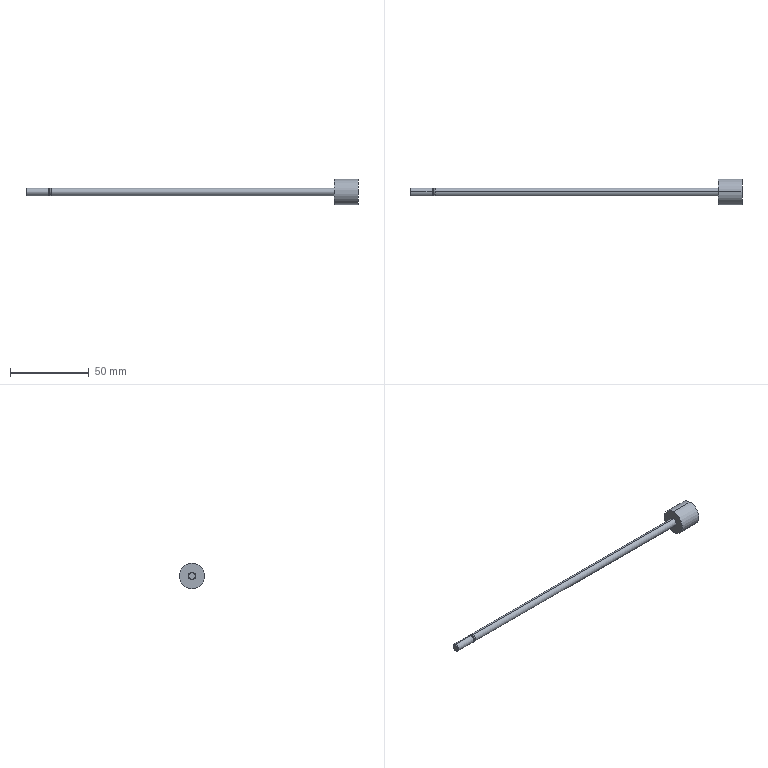Part | STEP file | QA-HI_SBA16x150-LB_R | 1 solid | 16 faces | box 210.5 x 16 x 16 mm | volume 6843 mm3 | cylinder 8 | cone 4 | plane 4 | commonest cylinder face diameters 5 x4 4 x2 16 x2
STEP:
#1=CARTESIAN_POINT('',(0.,0.,0.));
#2=DIRECTION('',(0.,0.,1.));
#3=DIRECTION('',(1.,0.,0.));
#4=AXIS2_PLACEMENT_3D('',#1,#2,#3);
#5=CARTESIAN_POINT('',(175.5,0.,2.5));
#6=VERTEX_POINT('',#5);
#7=CARTESIAN_POINT('',(175.5,0.,-2.5));
#8=VERTEX_POINT('',#7);
#9=CARTESIAN_POINT('',(175.5,0.,0.));
#10=DIRECTION('',(-1.,0.,0.));
#11=DIRECTION('',(0.,0.,1.));
#12=AXIS2_PLACEMENT_3D('',#9,#10,#11);
#13=CIRCLE('',#12,2.5);
#14=CARTESIAN_POINT('',(190.5,0.,0.));
#15=DIRECTION('',(-1.,0.,0.));
#16=DIRECTION('',(0.,0.,1.));
#17=AXIS2_PLACEMENT_3D('',#14,#15,#16);
#18=CYLINDRICAL_SURFACE('',#17,2.5);
#19=CARTESIAN_POINT('',(0.,15.));
#20=DIRECTION('',(1.,0.));
#21=VECTOR('',#20,1.);
#22=LINE('',#19,#21);
#23=(GEOMETRIC_REPRESENTATION_CONTEXT(2)PARAMETRIC_REPRESENTATION_CONTEXT()REPRESENTATION_CONTEXT('',''));
#24=DEFINITIONAL_REPRESENTATION('',(#22),#23);
#25=PCURVE('',#18,#24);
#26=CARTESIAN_POINT('',(175.5,2.5,0.));
#27=DIRECTION('',(1.,0.,0.));
#28=DIRECTION('',(0.,0.,-1.));
#29=AXIS2_PLACEMENT_3D('',#26,#27,#28);
#30=PLANE('',#29);
#31=CARTESIAN_POINT('',(-2.5,-2.5));
#32=CARTESIAN_POINT('',(-2.5,1.83));
#33=CARTESIAN_POINT('',(1.25,-0.3349));
#34=CARTESIAN_POINT('',(5.,-2.5));
#35=CARTESIAN_POINT('',(1.25,-4.665));
#36=CARTESIAN_POINT('',(-2.5,-6.83));
#37=CARTESIAN_POINT('',(-2.5,-2.5));
#38=(BOUNDED_CURVE()B_SPLINE_CURVE(2,(#31,#32,#33,#34,#35,#36,#37),.UNSPECIFIED.,.T.,.F.)B_SPLINE_CURVE_WITH_KNOTS((1,2,2,2,2,1),(-2.094,0.,2.094,4.189,6.283,8.378),.UNSPECIFIED.)CURVE()GEOMETRIC_REPRESENTATION_ITEM()RATIONAL_B_SPLINE_CURVE((1.,0.5,1.,0.5,1.,0.5,1.))REPRESENTATION_ITEM(''));
#39=(GEOMETRIC_REPRESENTATION_CONTEXT(2)PARAMETRIC_REPRESENTATION_CONTEXT()REPRESENTATION_CONTEXT('',''));
#40=DEFINITIONAL_REPRESENTATION('',(#38),#39);
#41=PCURVE('',#30,#40);
#42=SURFACE_CURVE('',#13,(#25,#41),.PCURVE_S1.);
#43=EDGE_CURVE('',#6,#8,#42,.T.);
#44=ORIENTED_EDGE('',*,*,#43,.T.);
#45=CARTESIAN_POINT('',(-4.134,0.,-2.5));
#46=VERTEX_POINT('',#45);
#47=CARTESIAN_POINT('',(190.5,0.,-2.5));
#48=DIRECTION('',(-1.,0.,0.));
#49=VECTOR('',#48,1.);
#50=LINE('',#47,#49);
#51=CARTESIAN_POINT('',(3.142,0.));
#52=DIRECTION('',(0.,1.));
#53=VECTOR('',#52,1.);
#54=LINE('',#51,#53);
#55=(GEOMETRIC_REPRESENTATION_CONTEXT(2)PARAMETRIC_REPRESENTATION_CONTEXT()REPRESENTATION_CONTEXT('',''));
#56=DEFINITIONAL_REPRESENTATION('',(#54),#55);
#57=PCURVE('',#18,#56);
#58=CARTESIAN_POINT('',(190.5,0.,0.));
#59=DIRECTION('',(-1.,0.,0.));
#60=DIRECTION('',(0.,0.,1.));
#61=AXIS2_PLACEMENT_3D('',#58,#59,#60);
#62=CYLINDRICAL_SURFACE('',#61,2.5);
#63=CARTESIAN_POINT('',(3.142,0.));
#64=DIRECTION('',(0.,1.));
#65=VECTOR('',#64,1.);
#66=LINE('',#63,#65);
#67=(GEOMETRIC_REPRESENTATION_CONTEXT(2)PARAMETRIC_REPRESENTATION_CONTEXT()REPRESENTATION_CONTEXT('',''));
#68=DEFINITIONAL_REPRESENTATION('',(#66),#67);
#69=PCURVE('',#62,#68);
#70=SURFACE_CURVE('',#50,(#57,#69),.PCURVE_S1.);
#71=EDGE_CURVE('',#8,#46,#70,.T.);
#72=ORIENTED_EDGE('',*,*,#71,.T.);
#73=CARTESIAN_POINT('',(-4.134,0.,2.5));
#74=VERTEX_POINT('',#73);
#75=CARTESIAN_POINT('',(-4.134,0.,0.));
#76=DIRECTION('',(1.,0.,0.));
#77=DIRECTION('',(0.,0.,1.));
#78=AXIS2_PLACEMENT_3D('',#75,#76,#77);
#79=CIRCLE('',#78,2.5);
#80=CARTESIAN_POINT('',(6.283,194.634));
#81=DIRECTION('',(-1.,0.));
#82=VECTOR('',#81,1.);
#83=LINE('',#80,#82);
#84=(GEOMETRIC_REPRESENTATION_CONTEXT(2)PARAMETRIC_REPRESENTATION_CONTEXT()REPRESENTATION_CONTEXT('',''));
#85=DEFINITIONAL_REPRESENTATION('',(#83),#84);
#86=PCURVE('',#18,#85);
#87=CARTESIAN_POINT('',(-4.134,0.,0.));
#88=DIRECTION('',(1.,0.,0.));
#89=DIRECTION('',(0.,0.,-1.));
#90=AXIS2_PLACEMENT_3D('',#87,#88,#89);
#91=CONICAL_SURFACE('',#90,2.5,0.5236);
#92=CARTESIAN_POINT('',(-3.142,0.));
#93=DIRECTION('',(1.,0.));
#94=VECTOR('',#93,1.);
#95=LINE('',#92,#94);
#96=(GEOMETRIC_REPRESENTATION_CONTEXT(2)PARAMETRIC_REPRESENTATION_CONTEXT()REPRESENTATION_CONTEXT('',''));
#97=DEFINITIONAL_REPRESENTATION('',(#95),#96);
#98=PCURVE('',#91,#97);
#99=SURFACE_CURVE('',#79,(#86,#98),.PCURVE_S1.);
#100=EDGE_CURVE('',#46,#74,#99,.T.);
#101=ORIENTED_EDGE('',*,*,#100,.T.);
#102=CARTESIAN_POINT('',(190.5,0.,2.5));
#103=DIRECTION('',(-1.,0.,0.));
#104=VECTOR('',#103,1.);
#105=LINE('',#102,#104);
#106=CARTESIAN_POINT('',(0.,0.));
#107=DIRECTION('',(0.,1.));
#108=VECTOR('',#107,1.);
#109=LINE('',#106,#108);
#110=(GEOMETRIC_REPRESENTATION_CONTEXT(2)PARAMETRIC_REPRESENTATION_CONTEXT()REPRESENTATION_CONTEXT('',''));
#111=DEFINITIONAL_REPRESENTATION('',(#109),#110);
#112=PCURVE('',#18,#111);
#113=CARTESIAN_POINT('',(6.283,0.));
#114=DIRECTION('',(0.,1.));
#115=VECTOR('',#114,1.);
#116=LINE('',#113,#115);
#117=(GEOMETRIC_REPRESENTATION_CONTEXT(2)PARAMETRIC_REPRESENTATION_CONTEXT()REPRESENTATION_CONTEXT('',''));
#118=DEFINITIONAL_REPRESENTATION('',(#116),#117);
#119=PCURVE('',#62,#118);
#120=SURFACE_CURVE('',#105,(#112,#119),.PCURVE_S1.);
#121=EDGE_CURVE('',#6,#74,#120,.T.);
#122=ORIENTED_EDGE('',*,*,#121,.F.);
#123=EDGE_LOOP('',(#44,#72,#101,#122));
#124=FACE_BOUND('',#123,.T.);
#125=ADVANCED_FACE('',(#124),#18,.T.);
#126=CARTESIAN_POINT('',(-5.,0.,-2.));
#127=VERTEX_POINT('',#126);
#128=CARTESIAN_POINT('',(-5.,0.,2.));
#129=VERTEX_POINT('',#128);
#130=CARTESIAN_POINT('',(-5.,0.,0.));
#131=DIRECTION('',(1.,0.,0.));
#132=DIRECTION('',(0.,0.,-1.));
#133=AXIS2_PLACEMENT_3D('',#130,#131,#132);
#134=CIRCLE('',#133,2.);
#135=CARTESIAN_POINT('',(0.,-0.866));
#136=DIRECTION('',(1.,0.));
#137=VECTOR('',#136,1.);
#138=LINE('',#135,#137);
#139=(GEOMETRIC_REPRESENTATION_CONTEXT(2)PARAMETRIC_REPRESENTATION_CONTEXT()REPRESENTATION_CONTEXT('',''));
#140=DEFINITIONAL_REPRESENTATION('',(#138),#139);
#141=PCURVE('',#91,#140);
#142=CARTESIAN_POINT('',(0.,0.,0.));
#143=DIRECTION('',(-1.,0.,0.));
#144=DIRECTION('',(0.,0.,1.));
#145=AXIS2_PLACEMENT_3D('',#142,#143,#144);
#146=CYLINDRICAL_SURFACE('',#145,2.);
#147=CARTESIAN_POINT('',(3.142,5.));
#148=DIRECTION('',(-1.,0.));
#149=VECTOR('',#148,1.);
#150=LINE('',#147,#149);
#151=(GEOMETRIC_REPRESENTATION_CONTEXT(2)PARAMETRIC_REPRESENTATION_CONTEXT()REPRESENTATION_CONTEXT('',''));
#152=DEFINITIONAL_REPRESENTATION('',(#150),#151);
#153=PCURVE('',#146,#152);
#154=SURFACE_CURVE('',#134,(#141,#153),.PCURVE_S1.);
#155=EDGE_CURVE('',#127,#129,#154,.T.);
#156=ORIENTED_EDGE('',*,*,#155,.T.);
#157=CARTESIAN_POINT('',(-4.134,0.,2.5));
#158=DIRECTION('',(0.866,0.,0.5));
#159=VECTOR('',#158,1.);
#160=LINE('',#157,#159);
#161=CARTESIAN_POINT('',(3.142,0.));
#162=DIRECTION('',(0.,1.));
#163=VECTOR('',#162,1.);
#164=LINE('',#161,#163);
#165=(GEOMETRIC_REPRESENTATION_CONTEXT(2)PARAMETRIC_REPRESENTATION_CONTEXT()REPRESENTATION_CONTEXT('',''));
#166=DEFINITIONAL_REPRESENTATION('',(#164),#165);
#167=PCURVE('',#91,#166);
#168=CARTESIAN_POINT('',(-4.134,0.,0.));
#169=DIRECTION('',(1.,0.,0.));
#170=DIRECTION('',(0.,0.,-1.));
#171=AXIS2_PLACEMENT_3D('',#168,#169,#170);
#172=CONICAL_SURFACE('',#171,2.5,0.5236);
#173=CARTESIAN_POINT('',(3.142,0.));
#174=DIRECTION('',(0.,1.));
#175=VECTOR('',#174,1.);
#176=LINE('',#173,#175);
#177=(GEOMETRIC_REPRESENTATION_CONTEXT(2)PARAMETRIC_REPRESENTATION_CONTEXT()REPRESENTATION_CONTEXT('',''));
#178=DEFINITIONAL_REPRESENTATION('',(#176),#177);
#179=PCURVE('',#172,#178);
#180=SURFACE_CURVE('',#160,(#167,#179),.PCURVE_S1.);
#181=EDGE_CURVE('',#129,#74,#180,.T.);
#182=ORIENTED_EDGE('',*,*,#181,.T.);
#183=ORIENTED_EDGE('',*,*,#100,.F.);
#184=CARTESIAN_POINT('',(-4.134,0.,-2.5));
#185=DIRECTION('',(0.866,0.,-0.5));
#186=VECTOR('',#185,1.);
#187=LINE('',#184,#186);
#188=CARTESIAN_POINT('',(0.,0.));
#189=DIRECTION('',(0.,1.));
#190=VECTOR('',#189,1.);
#191=LINE('',#188,#190);
#192=(GEOMETRIC_REPRESENTATION_CONTEXT(2)PARAMETRIC_REPRESENTATION_CONTEXT()REPRESENTATION_CONTEXT('',''));
#193=DEFINITIONAL_REPRESENTATION('',(#191),#192);
#194=PCURVE('',#91,#193);
#195=CARTESIAN_POINT('',(6.283,0.));
#196=DIRECTION('',(0.,1.));
#197=VECTOR('',#196,1.);
#198=LINE('',#195,#197);
#199=(GEOMETRIC_REPRESENTATION_CONTEXT(2)PARAMETRIC_REPRESENTATION_CONTEXT()REPRESENTATION_CONTEXT('',''));
#200=DEFINITIONAL_REPRESENTATION('',(#198),#199);
#201=PCURVE('',#172,#200);
#202=SURFACE_CURVE('',#187,(#194,#201),.PCURVE_S1.);
#203=EDGE_CURVE('',#127,#46,#202,.T.);
#204=ORIENTED_EDGE('',*,*,#203,.F.);
#205=EDGE_LOOP('',(#156,#182,#183,#204));
#206=FACE_BOUND('',#205,.T.);
#207=ADVANCED_FACE('',(#206),#91,.T.);
#208=ORIENTED_EDGE('',*,*,#155,.F.);
#209=CARTESIAN_POINT('',(-6.,0.,-2.));
#210=VERTEX_POINT('',#209);
#211=CARTESIAN_POINT('',(0.,0.,-2.));
#212=DIRECTION('',(-1.,0.,0.));
#213=VECTOR('',#212,1.);
#214=LINE('',#211,#213);
#215=CARTESIAN_POINT('',(3.142,0.));
#216=DIRECTION('',(0.,1.));
#217=VECTOR('',#216,1.);
#218=LINE('',#215,#217);
#219=(GEOMETRIC_REPRESENTATION_CONTEXT(2)PARAMETRIC_REPRESENTATION_CONTEXT()REPRESENTATION_CONTEXT('',''));
#220=DEFINITIONAL_REPRESENTATION('',(#218),#219);
#221=PCURVE('',#146,#220);
#222=CARTESIAN_POINT('',(0.,0.,0.));
#223=DIRECTION('',(-1.,0.,0.));
#224=DIRECTION('',(0.,0.,1.));
#225=AXIS2_PLACEMENT_3D('',#222,#223,#224);
#226=CYLINDRICAL_SURFACE('',#225,2.);
#227=CARTESIAN_POINT('',(3.142,0.));
#228=DIRECTION('',(0.,1.));
#229=VECTOR('',#228,1.);
#230=LINE('',#227,#229);
#231=(GEOMETRIC_REPRESENTATION_CONTEXT(2)PARAMETRIC_REPRESENTATION_CONTEXT()REPRESENTATION_CONTEXT('',''));
#232=DEFINITIONAL_REPRESENTATION('',(#230),#231);
#233=PCURVE('',#226,#232);
#234=SURFACE_CURVE('',#214,(#221,#233),.PCURVE_S1.);
#235=EDGE_CURVE('',#127,#210,#234,.T.);
#236=ORIENTED_EDGE('',*,*,#235,.T.);
#237=CARTESIAN_POINT('',(-6.,0.,2.));
#238=VERTEX_POINT('',#237);
#239=CARTESIAN_POINT('',(-6.,0.,0.));
#240=DIRECTION('',(1.,0.,0.));
#241=DIRECTION('',(0.,0.,1.));
#242=AXIS2_PLACEMENT_3D('',#239,#240,#241);
#243=CIRCLE('',#242,2.);
#244=CARTESIAN_POINT('',(6.283,6.));
#245=DIRECTION('',(-1.,0.));
#246=VECTOR('',#245,1.);
#247=LINE('',#244,#246);
#248=(GEOMETRIC_REPRESENTATION_CONTEXT(2)PARAMETRIC_REPRESENTATION_CONTEXT()REPRESENTATION_CONTEXT('',''));
#249=DEFINITIONAL_REPRESENTATION('',(#247),#248);
#250=PCURVE('',#146,#249);
#251=CARTESIAN_POINT('',(-6.,2.5,0.));
#252=DIRECTION('',(-1.,0.,0.));
#253=DIRECTION('',(0.,0.,1.));
#254=AXIS2_PLACEMENT_3D('',#251,#252,#253);
#255=PLANE('',#254);
#256=CARTESIAN_POINT('',(2.,-2.5));
#257=CARTESIAN_POINT('',(2.,-5.964));
#258=CARTESIAN_POINT('',(-1.,-4.232));
#259=CARTESIAN_POINT('',(-4.,-2.5));
#260=CARTESIAN_POINT('',(-1.,-0.7679));
#261=CARTESIAN_POINT('',(2.,0.9641));
#262=CARTESIAN_POINT('',(2.,-2.5));
#263=(BOUNDED_CURVE()B_SPLINE_CURVE(2,(#256,#257,#258,#259,#260,#261,#262),.UNSPECIFIED.,.T.,.F.)B_SPLINE_CURVE_WITH_KNOTS((1,2,2,2,2,1),(-2.094,0.,2.094,4.189,6.283,8.378),.UNSPECIFIED.)CURVE()GEOMETRIC_REPRESENTATION_ITEM()RATIONAL_B_SPLINE_CURVE((1.,0.5,1.,0.5,1.,0.5,1.))REPRESENTATION_ITEM(''));
#264=(GEOMETRIC_REPRESENTATION_CONTEXT(2)PARAMETRIC_REPRESENTATION_CONTEXT()REPRESENTATION_CONTEXT('',''));
#265=DEFINITIONAL_REPRESENTATION('',(#263),#264);
#266=PCURVE('',#255,#265);
#267=SURFACE_CURVE('',#243,(#250,#266),.PCURVE_S1.);
#268=EDGE_CURVE('',#210,#238,#267,.T.);
#269=ORIENTED_EDGE('',*,*,#268,.T.);
#270=CARTESIAN_POINT('',(0.,0.,2.));
#271=DIRECTION('',(-1.,0.,0.));
#272=VECTOR('',#271,1.);
#273=LINE('',#270,#272);
#274=CARTESIAN_POINT('',(0.,0.));
#275=DIRECTION('',(0.,1.));
#276=VECTOR('',#275,1.);
#277=LINE('',#274,#276);
#278=(GEOMETRIC_REPRESENTATION_CONTEXT(2)PARAMETRIC_REPRESENTATION_CONTEXT()REPRESENTATION_CONTEXT('',''));
#279=DEFINITIONAL_REPRESENTATION('',(#277),#278);
#280=PCURVE('',#146,#279);
#281=CARTESIAN_POINT('',(6.283,0.));
#282=DIRECTION('',(0.,1.));
#283=VECTOR('',#282,1.);
#284=LINE('',#281,#283);
#285=(GEOMETRIC_REPRESENTATION_CONTEXT(2)PARAMETRIC_REPRESENTATION_CONTEXT()REPRESENTATION_CONTEXT('',''));
#286=DEFINITIONAL_REPRESENTATION('',(#284),#285);
#287=PCURVE('',#226,#286);
#288=SURFACE_CURVE('',#273,(#280,#287),.PCURVE_S1.);
#289=EDGE_CURVE('',#129,#238,#288,.T.);
#290=ORIENTED_EDGE('',*,*,#289,.F.);
#291=EDGE_LOOP('',(#208,#236,#269,#290));
#292=FACE_BOUND('',#291,.T.);
#293=ADVANCED_FACE('',(#292),#146,.T.);
#294=CARTESIAN_POINT('',(190.5,0.,8.));
#295=VERTEX_POINT('',#294);
#296=CARTESIAN_POINT('',(190.5,0.,-8.));
#297=VERTEX_POINT('',#296);
#298=CARTESIAN_POINT('',(190.5,0.,0.));
#299=DIRECTION('',(-1.,0.,0.));
#300=DIRECTION('',(0.,0.,1.));
#301=AXIS2_PLACEMENT_3D('',#298,#299,#300);
#302=CIRCLE('',#301,8.);
#303=CARTESIAN_POINT('',(190.5,0.,0.));
#304=DIRECTION('',(-1.,0.,0.));
#305=DIRECTION('',(0.,0.,1.));
#306=AXIS2_PLACEMENT_3D('',#303,#304,#305);
#307=CYLINDRICAL_SURFACE('',#306,8.);
#308=CARTESIAN_POINT('',(0.,0.));
#309=DIRECTION('',(1.,0.));
#310=VECTOR('',#309,1.);
#311=LINE('',#308,#310);
#312=(GEOMETRIC_REPRESENTATION_CONTEXT(2)PARAMETRIC_REPRESENTATION_CONTEXT()REPRESENTATION_CONTEXT('',''));
#313=DEFINITIONAL_REPRESENTATION('',(#311),#312);
#314=PCURVE('',#307,#313);
#315=CARTESIAN_POINT('',(190.5,8.,0.));
#316=DIRECTION('',(-1.,0.,0.));
#317=DIRECTION('',(0.,0.,1.));
#318=AXIS2_PLACEMENT_3D('',#315,#316,#317);
#319=PLANE('',#318);
#320=CARTESIAN_POINT('',(0.,-8.));
#321=DIRECTION('',(1.,0.));
#322=AXIS2_PLACEMENT_2D('',#320,#321);
#323=CIRCLE('',#322,8.);
#324=(GEOMETRIC_REPRESENTATION_CONTEXT(2)PARAMETRIC_REPRESENTATION_CONTEXT()REPRESENTATION_CONTEXT('',''));
#325=DEFINITIONAL_REPRESENTATION('',(#323),#324);
#326=PCURVE('',#319,#325);
#327=SURFACE_CURVE('',#302,(#314,#326),.PCURVE_S1.);
#328=EDGE_CURVE('',#295,#297,#327,.T.);
#329=ORIENTED_EDGE('',*,*,#328,.T.);
#330=CARTESIAN_POINT('',(175.5,0.,-8.));
#331=VERTEX_POINT('',#330);
#332=CARTESIAN_POINT('',(190.5,0.,-8.));
#333=DIRECTION('',(-1.,0.,0.));
#334=VECTOR('',#333,1.);
#335=LINE('',#332,#334);
#336=CARTESIAN_POINT('',(3.142,0.));
#337=DIRECTION('',(0.,1.));
#338=VECTOR('',#337,1.);
#339=LINE('',#336,#338);
#340=(GEOMETRIC_REPRESENTATION_CONTEXT(2)PARAMETRIC_REPRESENTATION_CONTEXT()REPRESENTATION_CONTEXT('',''));
#341=DEFINITIONAL_REPRESENTATION('',(#339),#340);
#342=PCURVE('',#307,#341);
#343=CARTESIAN_POINT('',(190.5,0.,0.));
#344=DIRECTION('',(-1.,0.,0.));
#345=DIRECTION('',(0.,0.,1.));
#346=AXIS2_PLACEMENT_3D('',#343,#344,#345);
#347=CYLINDRICAL_SURFACE('',#346,8.);
#348=CARTESIAN_POINT('',(3.142,0.));
#349=DIRECTION('',(0.,1.));
#350=VECTOR('',#349,1.);
#351=LINE('',#348,#350);
#352=(GEOMETRIC_REPRESENTATION_CONTEXT(2)PARAMETRIC_REPRESENTATION_CONTEXT()REPRESENTATION_CONTEXT('',''));
#353=DEFINITIONAL_REPRESENTATION('',(#351),#352);
#354=PCURVE('',#347,#353);
#355=SURFACE_CURVE('',#335,(#342,#354),.PCURVE_S1.);
#356=EDGE_CURVE('',#297,#331,#355,.T.);
#357=ORIENTED_EDGE('',*,*,#356,.T.);
#358=CARTESIAN_POINT('',(175.5,0.,8.));
#359=VERTEX_POINT('',#358);
#360=CARTESIAN_POINT('',(175.5,0.,0.));
#361=DIRECTION('',(1.,0.,0.));
#362=DIRECTION('',(0.,0.,1.));
#363=AXIS2_PLACEMENT_3D('',#360,#361,#362);
#364=CIRCLE('',#363,8.);
#365=CARTESIAN_POINT('',(6.283,15.));
#366=DIRECTION('',(-1.,0.));
#367=VECTOR('',#366,1.);
#368=LINE('',#365,#367);
#369=(GEOMETRIC_REPRESENTATION_CONTEXT(2)PARAMETRIC_REPRESENTATION_CONTEXT()REPRESENTATION_CONTEXT('',''));
#370=DEFINITIONAL_REPRESENTATION('',(#368),#369);
#371=PCURVE('',#307,#370);
#372=CARTESIAN_POINT('',(0.,-2.5));
#373=DIRECTION('',(-1.,0.));
#374=AXIS2_PLACEMENT_2D('',#372,#373);
#375=CIRCLE('',#374,8.);
#376=(GEOMETRIC_REPRESENTATION_CONTEXT(2)PARAMETRIC_REPRESENTATION_CONTEXT()REPRESENTATION_CONTEXT('',''));
#377=DEFINITIONAL_REPRESENTATION('',(#375),#376);
#378=PCURVE('',#30,#377);
#379=SURFACE_CURVE('',#364,(#371,#378),.PCURVE_S1.);
#380=EDGE_CURVE('',#331,#359,#379,.T.);
#381=ORIENTED_EDGE('',*,*,#380,.T.);
#382=CARTESIAN_POINT('',(190.5,0.,8.));
#383=DIRECTION('',(-1.,0.,0.));
#384=VECTOR('',#383,1.);
#385=LINE('',#382,#384);
#386=CARTESIAN_POINT('',(0.,0.));
#387=DIRECTION('',(0.,1.));
#388=VECTOR('',#387,1.);
#389=LINE('',#386,#388);
#390=(GEOMETRIC_REPRESENTATION_CONTEXT(2)PARAMETRIC_REPRESENTATION_CONTEXT()REPRESENTATION_CONTEXT('',''));
#391=DEFINITIONAL_REPRESENTATION('',(#389),#390);
#392=PCURVE('',#307,#391);
#393=CARTESIAN_POINT('',(6.283,0.));
#394=DIRECTION('',(0.,1.));
#395=VECTOR('',#394,1.);
#396=LINE('',#393,#395);
#397=(GEOMETRIC_REPRESENTATION_CONTEXT(2)PARAMETRIC_REPRESENTATION_CONTEXT()REPRESENTATION_CONTEXT('',''));
#398=DEFINITIONAL_REPRESENTATION('',(#396),#397);
#399=PCURVE('',#347,#398);
#400=SURFACE_CURVE('',#385,(#392,#399),.PCURVE_S1.);
#401=EDGE_CURVE('',#295,#359,#400,.T.);
#402=ORIENTED_EDGE('',*,*,#401,.F.);
#403=EDGE_LOOP('',(#329,#357,#381,#402));
#404=FACE_BOUND('',#403,.T.);
#405=ADVANCED_FACE('',(#404),#307,.T.);
#406=CARTESIAN_POINT('',(-6.,0.,2.5));
#407=VERTEX_POINT('',#406);
#408=CARTESIAN_POINT('',(-6.,0.,-2.5));
#409=VERTEX_POINT('',#408);
#410=CARTESIAN_POINT('',(-6.,0.,0.));
#411=DIRECTION('',(-1.,0.,0.));
#412=DIRECTION('',(0.,0.,1.));
#413=AXIS2_PLACEMENT_3D('',#410,#411,#412);
#414=CIRCLE('',#413,2.5);
#415=CARTESIAN_POINT('',(0.,0.,0.));
#416=DIRECTION('',(-1.,0.,0.));
#417=DIRECTION('',(0.,0.,1.));
#418=AXIS2_PLACEMENT_3D('',#415,#416,#417);
#419=CYLINDRICAL_SURFACE('',#418,2.5);
#420=CARTESIAN_POINT('',(0.,6.));
#421=DIRECTION('',(1.,0.));
#422=VECTOR('',#421,1.);
#423=LINE('',#420,#422);
#424=(GEOMETRIC_REPRESENTATION_CONTEXT(2)PARAMETRIC_REPRESENTATION_CONTEXT()REPRESENTATION_CONTEXT('',''));
#425=DEFINITIONAL_REPRESENTATION('',(#423),#424);
#426=PCURVE('',#419,#425);
#427=CARTESIAN_POINT('',(0.,-2.5));
#428=DIRECTION('',(1.,0.));
#429=AXIS2_PLACEMENT_2D('',#427,#428);
#430=CIRCLE('',#429,2.5);
#431=(GEOMETRIC_REPRESENTATION_CONTEXT(2)PARAMETRIC_REPRESENTATION_CONTEXT()REPRESENTATION_CONTEXT('',''));
#432=DEFINITIONAL_REPRESENTATION('',(#430),#431);
#433=PCURVE('',#255,#432);
#434=SURFACE_CURVE('',#414,(#426,#433),.PCURVE_S1.);
#435=EDGE_CURVE('',#407,#409,#434,.T.);
#436=ORIENTED_EDGE('',*,*,#435,.T.);
#437=CARTESIAN_POINT('',(-19.509,0.,-2.5));
#438=VERTEX_POINT('',#437);
#439=CARTESIAN_POINT('',(0.,0.,-2.5));
#440=DIRECTION('',(-1.,0.,0.));
#441=VECTOR('',#440,1.);
#442=LINE('',#439,#441);
#443=CARTESIAN_POINT('',(3.142,0.));
#444=DIRECTION('',(0.,1.));
#445=VECTOR('',#444,1.);
#446=LINE('',#443,#445);
#447=(GEOMETRIC_REPRESENTATION_CONTEXT(2)PARAMETRIC_REPRESENTATION_CONTEXT()REPRESENTATION_CONTEXT('',''));
#448=DEFINITIONAL_REPRESENTATION('',(#446),#447);
#449=PCURVE('',#419,#448);
#450=CARTESIAN_POINT('',(0.,0.,0.));
#451=DIRECTION('',(-1.,0.,0.));
#452=DIRECTION('',(0.,0.,1.));
#453=AXIS2_PLACEMENT_3D('',#450,#451,#452);
#454=CYLINDRICAL_SURFACE('',#453,2.5);
#455=CARTESIAN_POINT('',(3.142,0.));
#456=DIRECTION('',(0.,1.));
#457=VECTOR('',#456,1.);
#458=LINE('',#455,#457);
#459=(GEOMETRIC_REPRESENTATION_CONTEXT(2)PARAMETRIC_REPRESENTATION_CONTEXT()REPRESENTATION_CONTEXT('',''));
#460=DEFINITIONAL_REPRESENTATION('',(#458),#459);
#461=PCURVE('',#454,#460);
#462=SURFACE_CURVE('',#442,(#449,#461),.PCURVE_S1.);
#463=EDGE_CURVE('',#409,#438,#462,.T.);
#464=ORIENTED_EDGE('',*,*,#463,.T.);
#465=CARTESIAN_POINT('',(-19.509,0.,2.5));
#466=VERTEX_POINT('',#465);
#467=CARTESIAN_POINT('',(-19.509,0.,0.));
#468=DIRECTION('',(1.,0.,0.));
#469=DIRECTION('',(0.,0.,1.));
#470=AXIS2_PLACEMENT_3D('',#467,#468,#469);
#471=CIRCLE('',#470,2.5);
#472=CARTESIAN_POINT('',(6.283,19.509));
#473=DIRECTION('',(-1.,0.));
#474=VECTOR('',#473,1.);
#475=LINE('',#472,#474);
#476=(GEOMETRIC_REPRESENTATION_CONTEXT(2)PARAMETRIC_REPRESENTATION_CONTEXT()REPRESENTATION_CONTEXT('',''));
#477=DEFINITIONAL_REPRESENTATION('',(#475),#476);
#478=PCURVE('',#419,#477);
#479=CARTESIAN_POINT('',(-19.51,0.,0.));
#480=DIRECTION('',(1.,0.,0.));
#481=DIRECTION('',(0.,0.,-1.));
#482=AXIS2_PLACEMENT_3D('',#479,#480,#481);
#483=CONICAL_SURFACE('',#482,2.5,0.7854);
#484=CARTESIAN_POINT('',(-3.142,0.));
#485=DIRECTION('',(1.,0.));
#486=VECTOR('',#485,1.);
#487=LINE('',#484,#486);
#488=(GEOMETRIC_REPRESENTATION_CONTEXT(2)PARAMETRIC_REPRESENTATION_CONTEXT()REPRESENTATION_CONTEXT('',''));
#489=DEFINITIONAL_REPRESENTATION('',(#487),#488);
#490=PCURVE('',#483,#489);
#491=SURFACE_CURVE('',#471,(#478,#490),.PCURVE_S1.);
#492=EDGE_CURVE('',#438,#466,#491,.T.);
#493=ORIENTED_EDGE('',*,*,#492,.T.);
#494=CARTESIAN_POINT('',(0.,0.,2.5));
#495=DIRECTION('',(-1.,0.,0.));
#496=VECTOR('',#495,1.);
#497=LINE('',#494,#496);
#498=CARTESIAN_POINT('',(0.,0.));
#499=DIRECTION('',(0.,1.));
#500=VECTOR('',#499,1.);
#501=LINE('',#498,#500);
#502=(GEOMETRIC_REPRESENTATION_CONTEXT(2)PARAMETRIC_REPRESENTATION_CONTEXT()REPRESENTATION_CONTEXT('',''));
#503=DEFINITIONAL_REPRESENTATION('',(#501),#502);
#504=PCURVE('',#419,#503);
#505=CARTESIAN_POINT('',(6.283,0.));
#506=DIRECTION('',(0.,1.));
#507=VECTOR('',#506,1.);
#508=LINE('',#505,#507);
#509=(GEOMETRIC_REPRESENTATION_CONTEXT(2)PARAMETRIC_REPRESENTATION_CONTEXT()REPRESENTATION_CONTEXT('',''));
#510=DEFINITIONAL_REPRESENTATION('',(#508),#509);
#511=PCURVE('',#454,#510);
#512=SURFACE_CURVE('',#497,(#504,#511),.PCURVE_S1.);
#513=EDGE_CURVE('',#407,#466,#512,.T.);
#514=ORIENTED_EDGE('',*,*,#513,.F.);
#515=EDGE_LOOP('',(#436,#464,#493,#514));
#516=FACE_BOUND('',#515,.T.);
#517=ADVANCED_FACE('',(#516),#419,.T.);
#518=CARTESIAN_POINT('',(-20.,0.,-2.009));
#519=VERTEX_POINT('',#518);
#520=CARTESIAN_POINT('',(-20.,0.,2.009));
#521=VERTEX_POINT('',#520);
#522=CARTESIAN_POINT('',(-20.,0.,0.));
#523=DIRECTION('',(1.,0.,0.));
#524=DIRECTION('',(0.,0.,-1.));
#525=AXIS2_PLACEMENT_3D('',#522,#523,#524);
#526=CIRCLE('',#525,2.009);
#527=CARTESIAN_POINT('',(0.,-0.4905));
#528=DIRECTION('',(1.,0.));
#529=VECTOR('',#528,1.);
#530=LINE('',#527,#529);
#531=(GEOMETRIC_REPRESENTATION_CONTEXT(2)PARAMETRIC_REPRESENTATION_CONTEXT()REPRESENTATION_CONTEXT('',''));
#532=DEFINITIONAL_REPRESENTATION('',(#530),#531);
#533=PCURVE('',#483,#532);
#534=CARTESIAN_POINT('',(-20.,0.,0.));
#535=DIRECTION('',(1.,0.,0.));
#536=DIRECTION('',(0.,0.,-1.));
#537=AXIS2_PLACEMENT_3D('',#534,#535,#536);
#538=PLANE('',#537);
#539=CARTESIAN_POINT('',(0.,0.));
#540=DIRECTION('',(1.,0.));
#541=AXIS2_PLACEMENT_2D('',#539,#540);
#542=CIRCLE('',#541,2.009);
#543=(GEOMETRIC_REPRESENTATION_CONTEXT(2)PARAMETRIC_REPRESENTATION_CONTEXT()REPRESENTATION_CONTEXT('',''));
#544=DEFINITIONAL_REPRESENTATION('',(#542),#543);
#545=PCURVE('',#538,#544);
#546=SURFACE_CURVE('',#526,(#533,#545),.PCURVE_S1.);
#547=EDGE_CURVE('',#519,#521,#546,.T.);
#548=ORIENTED_EDGE('',*,*,#547,.T.);
#549=CARTESIAN_POINT('',(-19.51,0.,2.5));
#550=DIRECTION('',(0.7071,0.,0.7071));
#551=VECTOR('',#550,1.);
#552=LINE('',#549,#551);
#553=CARTESIAN_POINT('',(3.142,0.));
#554=DIRECTION('',(0.,1.));
#555=VECTOR('',#554,1.);
#556=LINE('',#553,#555);
#557=(GEOMETRIC_REPRESENTATION_CONTEXT(2)PARAMETRIC_REPRESENTATION_CONTEXT()REPRESENTATION_CONTEXT('',''));
#558=DEFINITIONAL_REPRESENTATION('',(#556),#557);
#559=PCURVE('',#483,#558);
#560=CARTESIAN_POINT('',(-19.51,0.,0.));
#561=DIRECTION('',(1.,0.,0.));
#562=DIRECTION('',(0.,0.,-1.));
#563=AXIS2_PLACEMENT_3D('',#560,#561,#562);
#564=CONICAL_SURFACE('',#563,2.5,0.7854);
#565=CARTESIAN_POINT('',(3.142,0.));
#566=DIRECTION('',(0.,1.));
#567=VECTOR('',#566,1.);
#568=LINE('',#565,#567);
#569=(GEOMETRIC_REPRESENTATION_CONTEXT(2)PARAMETRIC_REPRESENTATION_CONTEXT()REPRESENTATION_CONTEXT('',''));
#570=DEFINITIONAL_REPRESENTATION('',(#568),#569);
#571=PCURVE('',#564,#570);
#572=SURFACE_CURVE('',#552,(#559,#571),.PCURVE_S1.);
#573=EDGE_CURVE('',#521,#466,#572,.T.);
#574=ORIENTED_EDGE('',*,*,#573,.T.);
#575=ORIENTED_EDGE('',*,*,#492,.F.);
#576=CARTESIAN_POINT('',(-19.51,0.,-2.5));
#577=DIRECTION('',(0.7071,0.,-0.7071));
#578=VECTOR('',#577,1.);
#579=LINE('',#576,#578);
#580=CARTESIAN_POINT('',(0.,0.));
#581=DIRECTION('',(0.,1.));
#582=VECTOR('',#581,1.);
#583=LINE('',#580,#582);
#584=(GEOMETRIC_REPRESENTATION_CONTEXT(2)PARAMETRIC_REPRESENTATION_CONTEXT()REPRESENTATION_CONTEXT('',''));
#585=DEFINITIONAL_REPRESENTATION('',(#583),#584);
#586=PCURVE('',#483,#585);
#587=CARTESIAN_POINT('',(6.283,0.));
#588=DIRECTION('',(0.,1.));
#589=VECTOR('',#588,1.);
#590=LINE('',#587,#589);
#591=(GEOMETRIC_REPRESENTATION_CONTEXT(2)PARAMETRIC_REPRESENTATION_CONTEXT()REPRESENTATION_CONTEXT('',''));
#592=DEFINITIONAL_REPRESENTATION('',(#590),#591);
#593=PCURVE('',#564,#592);
#594=SURFACE_CURVE('',#579,(#586,#593),.PCURVE_S1.);
#595=EDGE_CURVE('',#519,#438,#594,.T.);
#596=ORIENTED_EDGE('',*,*,#595,.F.);
#597=EDGE_LOOP('',(#548,#574,#575,#596));
#598=FACE_BOUND('',#597,.T.);
#599=ADVANCED_FACE('',(#598),#483,.T.);
#600=ORIENTED_EDGE('',*,*,#71,.F.);
#601=CARTESIAN_POINT('',(175.5,0.,0.));
#602=DIRECTION('',(-1.,0.,0.));
#603=DIRECTION('',(0.,0.,1.));
#604=AXIS2_PLACEMENT_3D('',#601,#602,#603);
#605=CIRCLE('',#604,2.5);
#606=CARTESIAN_POINT('',(0.,15.));
#607=DIRECTION('',(1.,0.));
#608=VECTOR('',#607,1.);
#609=LINE('',#606,#608);
#610=(GEOMETRIC_REPRESENTATION_CONTEXT(2)PARAMETRIC_REPRESENTATION_CONTEXT()REPRESENTATION_CONTEXT('',''));
#611=DEFINITIONAL_REPRESENTATION('',(#609),#610);
#612=PCURVE('',#62,#611);
#613=CARTESIAN_POINT('',(-2.5,-2.5));
#614=CARTESIAN_POINT('',(-2.5,1.83));
#615=CARTESIAN_POINT('',(1.25,-0.3349));
#616=CARTESIAN_POINT('',(5.,-2.5));
#617=CARTESIAN_POINT('',(1.25,-4.665));
#618=CARTESIAN_POINT('',(-2.5,-6.83));
#619=CARTESIAN_POINT('',(-2.5,-2.5));
#620=(BOUNDED_CURVE()B_SPLINE_CURVE(2,(#613,#614,#615,#616,#617,#618,#619),.UNSPECIFIED.,.T.,.F.)B_SPLINE_CURVE_WITH_KNOTS((1,2,2,2,2,1),(-2.094,0.,2.094,4.189,6.283,8.378),.UNSPECIFIED.)CURVE()GEOMETRIC_REPRESENTATION_ITEM()RATIONAL_B_SPLINE_CURVE((1.,0.5,1.,0.5,1.,0.5,1.))REPRESENTATION_ITEM(''));
#621=(GEOMETRIC_REPRESENTATION_CONTEXT(2)PARAMETRIC_REPRESENTATION_CONTEXT()REPRESENTATION_CONTEXT('',''));
#622=DEFINITIONAL_REPRESENTATION('',(#620),#621);
#623=PCURVE('',#30,#622);
#624=SURFACE_CURVE('',#605,(#612,#623),.PCURVE_S1.);
#625=EDGE_CURVE('',#8,#6,#624,.T.);
#626=ORIENTED_EDGE('',*,*,#625,.T.);
#627=ORIENTED_EDGE('',*,*,#121,.T.);
#628=CARTESIAN_POINT('',(-4.134,0.,0.));
#629=DIRECTION('',(1.,0.,0.));
#630=DIRECTION('',(0.,0.,1.));
#631=AXIS2_PLACEMENT_3D('',#628,#629,#630);
#632=CIRCLE('',#631,2.5);
#633=CARTESIAN_POINT('',(6.283,194.634));
#634=DIRECTION('',(-1.,0.));
#635=VECTOR('',#634,1.);
#636=LINE('',#633,#635);
#637=(GEOMETRIC_REPRESENTATION_CONTEXT(2)PARAMETRIC_REPRESENTATION_CONTEXT()REPRESENTATION_CONTEXT('',''));
#638=DEFINITIONAL_REPRESENTATION('',(#636),#637);
#639=PCURVE('',#62,#638);
#640=CARTESIAN_POINT('',(3.142,0.));
#641=DIRECTION('',(1.,0.));
#642=VECTOR('',#641,1.);
#643=LINE('',#640,#642);
#644=(GEOMETRIC_REPRESENTATION_CONTEXT(2)PARAMETRIC_REPRESENTATION_CONTEXT()REPRESENTATION_CONTEXT('',''));
#645=DEFINITIONAL_REPRESENTATION('',(#643),#644);
#646=PCURVE('',#172,#645);
#647=SURFACE_CURVE('',#632,(#639,#646),.PCURVE_S1.);
#648=EDGE_CURVE('',#74,#46,#647,.T.);
#649=ORIENTED_EDGE('',*,*,#648,.T.);
#650=EDGE_LOOP('',(#600,#626,#627,#649));
#651=FACE_BOUND('',#650,.T.);
#652=ADVANCED_FACE('',(#651),#62,.T.);
#653=ORIENTED_EDGE('',*,*,#181,.F.);
#654=CARTESIAN_POINT('',(-5.,0.,0.));
#655=DIRECTION('',(1.,0.,0.));
#656=DIRECTION('',(0.,0.,-1.));
#657=AXIS2_PLACEMENT_3D('',#654,#655,#656);
#658=CIRCLE('',#657,2.);
#659=CARTESIAN_POINT('',(0.,-0.866));
#660=DIRECTION('',(1.,0.));
#661=VECTOR('',#660,1.);
#662=LINE('',#659,#661);
#663=(GEOMETRIC_REPRESENTATION_CONTEXT(2)PARAMETRIC_REPRESENTATION_CONTEXT()REPRESENTATION_CONTEXT('',''));
#664=DEFINITIONAL_REPRESENTATION('',(#662),#663);
#665=PCURVE('',#172,#664);
#666=CARTESIAN_POINT('',(9.425,5.));
#667=DIRECTION('',(-1.,0.));
#668=VECTOR('',#667,1.);
#669=LINE('',#666,#668);
#670=(GEOMETRIC_REPRESENTATION_CONTEXT(2)PARAMETRIC_REPRESENTATION_CONTEXT()REPRESENTATION_CONTEXT('',''));
#671=DEFINITIONAL_REPRESENTATION('',(#669),#670);
#672=PCURVE('',#226,#671);
#673=SURFACE_CURVE('',#658,(#665,#672),.PCURVE_S1.);
#674=EDGE_CURVE('',#129,#127,#673,.T.);
#675=ORIENTED_EDGE('',*,*,#674,.T.);
#676=ORIENTED_EDGE('',*,*,#203,.T.);
#677=ORIENTED_EDGE('',*,*,#648,.F.);
#678=EDGE_LOOP('',(#653,#675,#676,#677));
#679=FACE_BOUND('',#678,.T.);
#680=ADVANCED_FACE('',(#679),#172,.T.);
#681=ORIENTED_EDGE('',*,*,#43,.F.);
#682=ORIENTED_EDGE('',*,*,#625,.F.);
#683=EDGE_LOOP('',(#681,#682));
#684=FACE_BOUND('',#683,.T.);
#685=CARTESIAN_POINT('',(175.5,0.,0.));
#686=DIRECTION('',(1.,0.,0.));
#687=DIRECTION('',(0.,0.,1.));
#688=AXIS2_PLACEMENT_3D('',#685,#686,#687);
#689=CIRCLE('',#688,8.);
#690=CARTESIAN_POINT('',(0.,-2.5));
#691=DIRECTION('',(-1.,0.));
#692=AXIS2_PLACEMENT_2D('',#690,#691);
#693=CIRCLE('',#692,8.);
#694=(GEOMETRIC_REPRESENTATION_CONTEXT(2)PARAMETRIC_REPRESENTATION_CONTEXT()REPRESENTATION_CONTEXT('',''));
#695=DEFINITIONAL_REPRESENTATION('',(#693),#694);
#696=PCURVE('',#30,#695);
#697=CARTESIAN_POINT('',(6.283,15.));
#698=DIRECTION('',(-1.,0.));
#699=VECTOR('',#698,1.);
#700=LINE('',#697,#699);
#701=(GEOMETRIC_REPRESENTATION_CONTEXT(2)PARAMETRIC_REPRESENTATION_CONTEXT()REPRESENTATION_CONTEXT('',''));
#702=DEFINITIONAL_REPRESENTATION('',(#700),#701);
#703=PCURVE('',#347,#702);
#704=SURFACE_CURVE('',#689,(#696,#703),.PCURVE_S1.);
#705=EDGE_CURVE('',#359,#331,#704,.T.);
#706=ORIENTED_EDGE('',*,*,#705,.F.);
#707=ORIENTED_EDGE('',*,*,#380,.F.);
#708=EDGE_LOOP('',(#706,#707));
#709=FACE_BOUND('',#708,.T.);
#710=ADVANCED_FACE('',(#684,#709),#30,.F.);
#711=ORIENTED_EDGE('',*,*,#235,.F.);
#712=ORIENTED_EDGE('',*,*,#674,.F.);
#713=ORIENTED_EDGE('',*,*,#289,.T.);
#714=CARTESIAN_POINT('',(-6.,0.,0.));
#715=DIRECTION('',(1.,0.,0.));
#716=DIRECTION('',(0.,0.,1.));
#717=AXIS2_PLACEMENT_3D('',#714,#715,#716);
#718=CIRCLE('',#717,2.);
#719=CARTESIAN_POINT('',(6.283,6.));
#720=DIRECTION('',(-1.,0.));
#721=VECTOR('',#720,1.);
#722=LINE('',#719,#721);
#723=(GEOMETRIC_REPRESENTATION_CONTEXT(2)PARAMETRIC_REPRESENTATION_CONTEXT()REPRESENTATION_CONTEXT('',''));
#724=DEFINITIONAL_REPRESENTATION('',(#722),#723);
#725=PCURVE('',#226,#724);
#726=CARTESIAN_POINT('',(2.,-2.5));
#727=CARTESIAN_POINT('',(2.,-5.964));
#728=CARTESIAN_POINT('',(-1.,-4.232));
#729=CARTESIAN_POINT('',(-4.,-2.5));
#730=CARTESIAN_POINT('',(-1.,-0.7679));
#731=CARTESIAN_POINT('',(2.,0.9641));
#732=CARTESIAN_POINT('',(2.,-2.5));
#733=(BOUNDED_CURVE()B_SPLINE_CURVE(2,(#726,#727,#728,#729,#730,#731,#732),.UNSPECIFIED.,.T.,.F.)B_SPLINE_CURVE_WITH_KNOTS((1,2,2,2,2,1),(-2.094,0.,2.094,4.189,6.283,8.378),.UNSPECIFIED.)CURVE()GEOMETRIC_REPRESENTATION_ITEM()RATIONAL_B_SPLINE_CURVE((1.,0.5,1.,0.5,1.,0.5,1.))REPRESENTATION_ITEM(''));
#734=(GEOMETRIC_REPRESENTATION_CONTEXT(2)PARAMETRIC_REPRESENTATION_CONTEXT()REPRESENTATION_CONTEXT('',''));
#735=DEFINITIONAL_REPRESENTATION('',(#733),#734);
#736=PCURVE('',#255,#735);
#737=SURFACE_CURVE('',#718,(#725,#736),.PCURVE_S1.);
#738=EDGE_CURVE('',#238,#210,#737,.T.);
#739=ORIENTED_EDGE('',*,*,#738,.T.);
#740=EDGE_LOOP('',(#711,#712,#713,#739));
#741=FACE_BOUND('',#740,.T.);
#742=ADVANCED_FACE('',(#741),#226,.T.);
#743=ORIENTED_EDGE('',*,*,#356,.F.);
#744=CARTESIAN_POINT('',(190.5,0.,0.));
#745=DIRECTION('',(-1.,0.,0.));
#746=DIRECTION('',(0.,0.,1.));
#747=AXIS2_PLACEMENT_3D('',#744,#745,#746);
#748=CIRCLE('',#747,8.);
#749=CARTESIAN_POINT('',(0.,0.));
#750=DIRECTION('',(1.,0.));
#751=VECTOR('',#750,1.);
#752=LINE('',#749,#751);
#753=(GEOMETRIC_REPRESENTATION_CONTEXT(2)PARAMETRIC_REPRESENTATION_CONTEXT()REPRESENTATION_CONTEXT('',''));
#754=DEFINITIONAL_REPRESENTATION('',(#752),#753);
#755=PCURVE('',#347,#754);
#756=CARTESIAN_POINT('',(0.,-8.));
#757=DIRECTION('',(1.,0.));
#758=AXIS2_PLACEMENT_2D('',#756,#757);
#759=CIRCLE('',#758,8.);
#760=(GEOMETRIC_REPRESENTATION_CONTEXT(2)PARAMETRIC_REPRESENTATION_CONTEXT()REPRESENTATION_CONTEXT('',''));
#761=DEFINITIONAL_REPRESENTATION('',(#759),#760);
#762=PCURVE('',#319,#761);
#763=SURFACE_CURVE('',#748,(#755,#762),.PCURVE_S1.);
#764=EDGE_CURVE('',#297,#295,#763,.T.);
#765=ORIENTED_EDGE('',*,*,#764,.T.);
#766=ORIENTED_EDGE('',*,*,#401,.T.);
#767=ORIENTED_EDGE('',*,*,#705,.T.);
#768=EDGE_LOOP('',(#743,#765,#766,#767));
#769=FACE_BOUND('',#768,.T.);
#770=ADVANCED_FACE('',(#769),#347,.T.);
#771=ORIENTED_EDGE('',*,*,#435,.F.);
#772=CARTESIAN_POINT('',(-6.,0.,0.));
#773=DIRECTION('',(-1.,0.,0.));
#774=DIRECTION('',(0.,0.,1.));
#775=AXIS2_PLACEMENT_3D('',#772,#773,#774);
#776=CIRCLE('',#775,2.5);
#777=CARTESIAN_POINT('',(0.,-2.5));
#778=DIRECTION('',(1.,0.));
#779=AXIS2_PLACEMENT_2D('',#777,#778);
#780=CIRCLE('',#779,2.5);
#781=(GEOMETRIC_REPRESENTATION_CONTEXT(2)PARAMETRIC_REPRESENTATION_CONTEXT()REPRESENTATION_CONTEXT('',''));
#782=DEFINITIONAL_REPRESENTATION('',(#780),#781);
#783=PCURVE('',#255,#782);
#784=CARTESIAN_POINT('',(0.,6.));
#785=DIRECTION('',(1.,0.));
#786=VECTOR('',#785,1.);
#787=LINE('',#784,#786);
#788=(GEOMETRIC_REPRESENTATION_CONTEXT(2)PARAMETRIC_REPRESENTATION_CONTEXT()REPRESENTATION_CONTEXT('',''));
#789=DEFINITIONAL_REPRESENTATION('',(#787),#788);
#790=PCURVE('',#454,#789);
#791=SURFACE_CURVE('',#776,(#783,#790),.PCURVE_S1.);
#792=EDGE_CURVE('',#409,#407,#791,.T.);
#793=ORIENTED_EDGE('',*,*,#792,.F.);
#794=EDGE_LOOP('',(#771,#793));
#795=FACE_BOUND('',#794,.T.);
#796=ORIENTED_EDGE('',*,*,#738,.F.);
#797=ORIENTED_EDGE('',*,*,#268,.F.);
#798=EDGE_LOOP('',(#796,#797));
#799=FACE_BOUND('',#798,.T.);
#800=ADVANCED_FACE('',(#795,#799),#255,.F.);
#801=ORIENTED_EDGE('',*,*,#328,.F.);
#802=ORIENTED_EDGE('',*,*,#764,.F.);
#803=EDGE_LOOP('',(#801,#802));
#804=FACE_BOUND('',#803,.T.);
#805=ADVANCED_FACE('',(#804),#319,.F.);
#806=ORIENTED_EDGE('',*,*,#463,.F.);
#807=ORIENTED_EDGE('',*,*,#792,.T.);
#808=ORIENTED_EDGE('',*,*,#513,.T.);
#809=CARTESIAN_POINT('',(-19.509,0.,0.));
#810=DIRECTION('',(1.,0.,0.));
#811=DIRECTION('',(0.,0.,1.));
#812=AXIS2_PLACEMENT_3D('',#809,#810,#811);
#813=CIRCLE('',#812,2.5);
#814=CARTESIAN_POINT('',(6.283,19.509));
#815=DIRECTION('',(-1.,0.));
#816=VECTOR('',#815,1.);
#817=LINE('',#814,#816);
#818=(GEOMETRIC_REPRESENTATION_CONTEXT(2)PARAMETRIC_REPRESENTATION_CONTEXT()REPRESENTATION_CONTEXT('',''));
#819=DEFINITIONAL_REPRESENTATION('',(#817),#818);
#820=PCURVE('',#454,#819);
#821=CARTESIAN_POINT('',(3.142,0.));
#822=DIRECTION('',(1.,0.));
#823=VECTOR('',#822,1.);
#824=LINE('',#821,#823);
#825=(GEOMETRIC_REPRESENTATION_CONTEXT(2)PARAMETRIC_REPRESENTATION_CONTEXT()REPRESENTATION_CONTEXT('',''));
#826=DEFINITIONAL_REPRESENTATION('',(#824),#825);
#827=PCURVE('',#564,#826);
#828=SURFACE_CURVE('',#813,(#820,#827),.PCURVE_S1.);
#829=EDGE_CURVE('',#466,#438,#828,.T.);
#830=ORIENTED_EDGE('',*,*,#829,.T.);
#831=EDGE_LOOP('',(#806,#807,#808,#830));
#832=FACE_BOUND('',#831,.T.);
#833=ADVANCED_FACE('',(#832),#454,.T.);
#834=ORIENTED_EDGE('',*,*,#573,.F.);
#835=CARTESIAN_POINT('',(-20.,0.,0.));
#836=DIRECTION('',(1.,0.,0.));
#837=DIRECTION('',(0.,0.,-1.));
#838=AXIS2_PLACEMENT_3D('',#835,#836,#837);
#839=CIRCLE('',#838,2.009);
#840=CARTESIAN_POINT('',(0.,-0.4905));
#841=DIRECTION('',(1.,0.));
#842=VECTOR('',#841,1.);
#843=LINE('',#840,#842);
#844=(GEOMETRIC_REPRESENTATION_CONTEXT(2)PARAMETRIC_REPRESENTATION_CONTEXT()REPRESENTATION_CONTEXT('',''));
#845=DEFINITIONAL_REPRESENTATION('',(#843),#844);
#846=PCURVE('',#564,#845);
#847=CARTESIAN_POINT('',(0.,0.));
#848=DIRECTION('',(1.,0.));
#849=AXIS2_PLACEMENT_2D('',#847,#848);
#850=CIRCLE('',#849,2.009);
#851=(GEOMETRIC_REPRESENTATION_CONTEXT(2)PARAMETRIC_REPRESENTATION_CONTEXT()REPRESENTATION_CONTEXT('',''));
#852=DEFINITIONAL_REPRESENTATION('',(#850),#851);
#853=PCURVE('',#538,#852);
#854=SURFACE_CURVE('',#839,(#846,#853),.PCURVE_S1.);
#855=EDGE_CURVE('',#521,#519,#854,.T.);
#856=ORIENTED_EDGE('',*,*,#855,.T.);
#857=ORIENTED_EDGE('',*,*,#595,.T.);
#858=ORIENTED_EDGE('',*,*,#829,.F.);
#859=EDGE_LOOP('',(#834,#856,#857,#858));
#860=FACE_BOUND('',#859,.T.);
#861=ADVANCED_FACE('',(#860),#564,.T.);
#862=ORIENTED_EDGE('',*,*,#547,.F.);
#863=ORIENTED_EDGE('',*,*,#855,.F.);
#864=EDGE_LOOP('',(#862,#863));
#865=FACE_BOUND('',#864,.T.);
#866=ADVANCED_FACE('',(#865),#538,.F.);
#867=CLOSED_SHELL('',(#125,#207,#293,#405,#517,#599,#652,#680,#710,#742,#770,#800,#805,#833,#861,#866));
#868=MANIFOLD_SOLID_BREP('',#867);
#869=(LENGTH_UNIT()NAMED_UNIT(*)SI_UNIT(.MILLI.,.METRE.));
#870=UNCERTAINTY_MEASURE_WITH_UNIT(LENGTH_MEASURE(0.0000001),#869,'','');
#871=(NAMED_UNIT(*)PLANE_ANGLE_UNIT()SI_UNIT($,.RADIAN.));
#872=(NAMED_UNIT(*)SI_UNIT($,.STERADIAN.)SOLID_ANGLE_UNIT());
#873=(GEOMETRIC_REPRESENTATION_CONTEXT(3)GLOBAL_UNCERTAINTY_ASSIGNED_CONTEXT((#870))GLOBAL_UNIT_ASSIGNED_CONTEXT((#869,#871,#872))REPRESENTATION_CONTEXT('',''));
#874=ADVANCED_BREP_SHAPE_REPRESENTATION('',(#4,#868),#873);